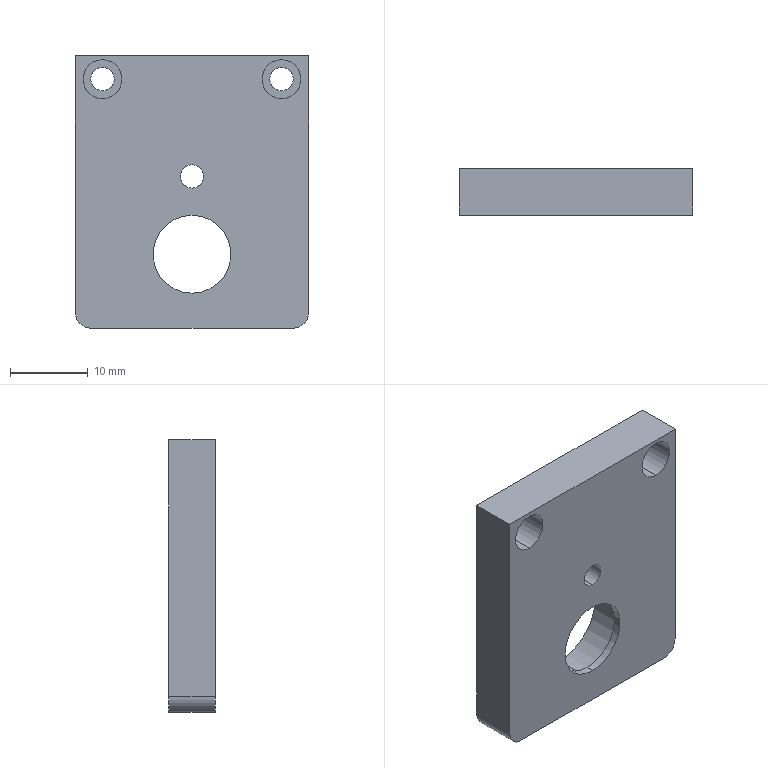Part | SolidWorks | features ICE 4, Cut 2, Extrusion 1, HoleWzd 1 | 1 solid | 33 faces | box 30 x 6 x 35 mm | volume 5244 mm3 | cylinder 20 | plane 9 | cone 4 | commonest cylinder face diameters 3 x6 2.5 x4 5 x4 4 x2 10 x2 13 x2
STEP:
#1=CARTESIAN_POINT('',(7.5,3.,3.25));
#2=VERTEX_POINT('',#1);
#3=CARTESIAN_POINT('',(7.5,3.,0.75));
#4=VERTEX_POINT('',#3);
#5=CARTESIAN_POINT('',(7.5,3.,2.));
#6=DIRECTION('',(1.,0.,0.));
#7=DIRECTION('',(0.,0.,-1.));
#8=AXIS2_PLACEMENT_3D('',#5,#6,#7);
#9=CIRCLE('',#8,1.25);
#10=EDGE_CURVE('',#2,#4,#9,.T.);
#11=ORIENTED_EDGE('',*,*,#10,.F.);
#12=CARTESIAN_POINT('',(15.,3.,3.25));
#13=VERTEX_POINT('',#12);
#14=CARTESIAN_POINT('',(15.,3.,3.25));
#15=DIRECTION('',(1.,0.,0.));
#16=VECTOR('',#15,1000.);
#17=LINE('',#14,#16);
#18=EDGE_CURVE('',#2,#13,#17,.T.);
#19=ORIENTED_EDGE('',*,*,#18,.T.);
#20=CARTESIAN_POINT('',(15.,3.,0.75));
#21=VERTEX_POINT('',#20);
#22=CARTESIAN_POINT('',(15.,3.,2.));
#23=DIRECTION('',(1.,0.,0.));
#24=DIRECTION('',(0.,0.,-1.));
#25=AXIS2_PLACEMENT_3D('',#22,#23,#24);
#26=CIRCLE('',#25,1.25);
#27=EDGE_CURVE('',#13,#21,#26,.T.);
#28=ORIENTED_EDGE('',*,*,#27,.T.);
#29=CARTESIAN_POINT('',(15.,3.,0.75));
#30=DIRECTION('',(1.,0.,0.));
#31=VECTOR('',#30,1000.);
#32=LINE('',#29,#31);
#33=EDGE_CURVE('',#4,#21,#32,.T.);
#34=ORIENTED_EDGE('',*,*,#33,.F.);
#35=EDGE_LOOP('',(#11,#19,#28,#34));
#36=FACE_OUTER_BOUND('',#35,.T.);
#37=CARTESIAN_POINT('',(15.,3.,2.));
#38=DIRECTION('',(1.,0.,0.));
#39=DIRECTION('',(0.,0.,-1.));
#40=AXIS2_PLACEMENT_3D('',#37,#38,#39);
#41=CYLINDRICAL_SURFACE('',#40,1.25);
#42=ADVANCED_FACE('',(#36),#41,.F.);
#43=CARTESIAN_POINT('',(6.749,3.,2.));
#44=VERTEX_POINT('',#43);
#45=CARTESIAN_POINT('',(7.5,3.,0.75));
#46=DIRECTION('',(0.515,0.,-0.8572));
#47=VECTOR('',#46,1000.);
#48=LINE('',#45,#47);
#49=EDGE_CURVE('',#44,#4,#48,.T.);
#50=ORIENTED_EDGE('',*,*,#49,.F.);
#51=CARTESIAN_POINT('',(7.5,3.,3.25));
#52=DIRECTION('',(0.515,0.,0.8572));
#53=VECTOR('',#52,1000.);
#54=LINE('',#51,#53);
#55=EDGE_CURVE('',#44,#2,#54,.T.);
#56=ORIENTED_EDGE('',*,*,#55,.T.);
#57=ORIENTED_EDGE('',*,*,#10,.T.);
#58=EDGE_LOOP('',(#50,#56,#57));
#59=FACE_OUTER_BOUND('',#58,.T.);
#60=CARTESIAN_POINT('',(7.5,3.,2.));
#61=DIRECTION('',(1.,0.,0.));
#62=DIRECTION('',(0.,0.,-1.));
#63=AXIS2_PLACEMENT_3D('',#60,#61,#62);
#64=CONICAL_SURFACE('',#63,1.25,1.03);
#65=ADVANCED_FACE('',(#59),#64,.F.);
#66=CARTESIAN_POINT('',(7.5,3.,-6.25));
#67=VERTEX_POINT('',#66);
#68=CARTESIAN_POINT('',(7.5,3.,-8.75));
#69=VERTEX_POINT('',#68);
#70=CARTESIAN_POINT('',(7.5,3.,-7.5));
#71=DIRECTION('',(1.,0.,0.));
#72=DIRECTION('',(0.,0.,-1.));
#73=AXIS2_PLACEMENT_3D('',#70,#71,#72);
#74=CIRCLE('',#73,1.25);
#75=EDGE_CURVE('',#67,#69,#74,.T.);
#76=ORIENTED_EDGE('',*,*,#75,.F.);
#77=CARTESIAN_POINT('',(15.,3.,-6.25));
#78=VERTEX_POINT('',#77);
#79=CARTESIAN_POINT('',(15.,3.,-6.25));
#80=DIRECTION('',(1.,0.,0.));
#81=VECTOR('',#80,1000.);
#82=LINE('',#79,#81);
#83=EDGE_CURVE('',#67,#78,#82,.T.);
#84=ORIENTED_EDGE('',*,*,#83,.T.);
#85=CARTESIAN_POINT('',(15.,3.,-8.75));
#86=VERTEX_POINT('',#85);
#87=CARTESIAN_POINT('',(15.,3.,-7.5));
#88=DIRECTION('',(1.,0.,0.));
#89=DIRECTION('',(0.,0.,-1.));
#90=AXIS2_PLACEMENT_3D('',#87,#88,#89);
#91=CIRCLE('',#90,1.25);
#92=EDGE_CURVE('',#78,#86,#91,.T.);
#93=ORIENTED_EDGE('',*,*,#92,.T.);
#94=CARTESIAN_POINT('',(15.,3.,-8.75));
#95=DIRECTION('',(1.,0.,0.));
#96=VECTOR('',#95,1000.);
#97=LINE('',#94,#96);
#98=EDGE_CURVE('',#69,#86,#97,.T.);
#99=ORIENTED_EDGE('',*,*,#98,.F.);
#100=EDGE_LOOP('',(#76,#84,#93,#99));
#101=FACE_OUTER_BOUND('',#100,.T.);
#102=CARTESIAN_POINT('',(15.,3.,-7.5));
#103=DIRECTION('',(1.,0.,0.));
#104=DIRECTION('',(0.,0.,-1.));
#105=AXIS2_PLACEMENT_3D('',#102,#103,#104);
#106=CYLINDRICAL_SURFACE('',#105,1.25);
#107=ADVANCED_FACE('',(#101),#106,.F.);
#108=CARTESIAN_POINT('',(6.749,3.,-7.5));
#109=VERTEX_POINT('',#108);
#110=CARTESIAN_POINT('',(7.5,3.,-8.75));
#111=DIRECTION('',(0.515,0.,-0.8572));
#112=VECTOR('',#111,1000.);
#113=LINE('',#110,#112);
#114=EDGE_CURVE('',#109,#69,#113,.T.);
#115=ORIENTED_EDGE('',*,*,#114,.F.);
#116=CARTESIAN_POINT('',(7.5,3.,-6.25));
#117=DIRECTION('',(0.515,0.,0.8572));
#118=VECTOR('',#117,1000.);
#119=LINE('',#116,#118);
#120=EDGE_CURVE('',#109,#67,#119,.T.);
#121=ORIENTED_EDGE('',*,*,#120,.T.);
#122=ORIENTED_EDGE('',*,*,#75,.T.);
#123=EDGE_LOOP('',(#115,#121,#122));
#124=FACE_OUTER_BOUND('',#123,.T.);
#125=CARTESIAN_POINT('',(7.5,3.,-7.5));
#126=DIRECTION('',(1.,0.,0.));
#127=DIRECTION('',(0.,0.,-1.));
#128=AXIS2_PLACEMENT_3D('',#125,#126,#127);
#129=CONICAL_SURFACE('',#128,1.25,1.03);
#130=ADVANCED_FACE('',(#124),#129,.F.);
#131=CARTESIAN_POINT('',(11.5,4.,17.));
#132=VERTEX_POINT('',#131);
#133=CARTESIAN_POINT('',(11.5,4.,12.));
#134=VERTEX_POINT('',#133);
#135=CARTESIAN_POINT('',(11.5,4.,14.5));
#136=DIRECTION('',(0.,-1.,0.));
#137=DIRECTION('',(0.,0.,-1.));
#138=AXIS2_PLACEMENT_3D('',#135,#136,#137);
#139=CIRCLE('',#138,2.5);
#140=EDGE_CURVE('',#132,#134,#139,.T.);
#141=ORIENTED_EDGE('',*,*,#140,.F.);
#142=CARTESIAN_POINT('',(11.5,0.,17.));
#143=VERTEX_POINT('',#142);
#144=CARTESIAN_POINT('',(11.5,4.,17.));
#145=DIRECTION('',(0.,-1.,0.));
#146=VECTOR('',#145,1000.);
#147=LINE('',#144,#146);
#148=EDGE_CURVE('',#132,#143,#147,.T.);
#149=ORIENTED_EDGE('',*,*,#148,.T.);
#150=CARTESIAN_POINT('',(11.5,0.,12.));
#151=VERTEX_POINT('',#150);
#152=CARTESIAN_POINT('',(11.5,0.,14.5));
#153=DIRECTION('',(0.,-1.,0.));
#154=DIRECTION('',(0.,0.,-1.));
#155=AXIS2_PLACEMENT_3D('',#152,#153,#154);
#156=CIRCLE('',#155,2.5);
#157=EDGE_CURVE('',#143,#151,#156,.T.);
#158=ORIENTED_EDGE('',*,*,#157,.T.);
#159=CARTESIAN_POINT('',(11.5,4.,12.));
#160=DIRECTION('',(0.,-1.,0.));
#161=VECTOR('',#160,1000.);
#162=LINE('',#159,#161);
#163=EDGE_CURVE('',#134,#151,#162,.T.);
#164=ORIENTED_EDGE('',*,*,#163,.F.);
#165=EDGE_LOOP('',(#141,#149,#158,#164));
#166=FACE_OUTER_BOUND('',#165,.T.);
#167=CARTESIAN_POINT('',(11.5,4.,14.5));
#168=DIRECTION('',(0.,-1.,0.));
#169=DIRECTION('',(0.,0.,-1.));
#170=AXIS2_PLACEMENT_3D('',#167,#168,#169);
#171=CYLINDRICAL_SURFACE('',#170,2.5);
#172=ADVANCED_FACE('',(#166),#171,.F.);
#173=CARTESIAN_POINT('',(-11.5,4.,17.));
#174=VERTEX_POINT('',#173);
#175=CARTESIAN_POINT('',(-11.5,4.,12.));
#176=VERTEX_POINT('',#175);
#177=CARTESIAN_POINT('',(-11.5,4.,14.5));
#178=DIRECTION('',(0.,-1.,0.));
#179=DIRECTION('',(0.,0.,-1.));
#180=AXIS2_PLACEMENT_3D('',#177,#178,#179);
#181=CIRCLE('',#180,2.5);
#182=EDGE_CURVE('',#174,#176,#181,.T.);
#183=ORIENTED_EDGE('',*,*,#182,.F.);
#184=CARTESIAN_POINT('',(-11.5,0.,17.));
#185=VERTEX_POINT('',#184);
#186=CARTESIAN_POINT('',(-11.5,4.,17.));
#187=DIRECTION('',(0.,-1.,0.));
#188=VECTOR('',#187,1000.);
#189=LINE('',#186,#188);
#190=EDGE_CURVE('',#174,#185,#189,.T.);
#191=ORIENTED_EDGE('',*,*,#190,.T.);
#192=CARTESIAN_POINT('',(-11.5,0.,12.));
#193=VERTEX_POINT('',#192);
#194=CARTESIAN_POINT('',(-11.5,0.,14.5));
#195=DIRECTION('',(0.,-1.,0.));
#196=DIRECTION('',(0.,0.,-1.));
#197=AXIS2_PLACEMENT_3D('',#194,#195,#196);
#198=CIRCLE('',#197,2.5);
#199=EDGE_CURVE('',#185,#193,#198,.T.);
#200=ORIENTED_EDGE('',*,*,#199,.T.);
#201=CARTESIAN_POINT('',(-11.5,4.,12.));
#202=DIRECTION('',(0.,-1.,0.));
#203=VECTOR('',#202,1000.);
#204=LINE('',#201,#203);
#205=EDGE_CURVE('',#176,#193,#204,.T.);
#206=ORIENTED_EDGE('',*,*,#205,.F.);
#207=EDGE_LOOP('',(#183,#191,#200,#206));
#208=FACE_OUTER_BOUND('',#207,.T.);
#209=CARTESIAN_POINT('',(-11.5,4.,14.5));
#210=DIRECTION('',(0.,-1.,0.));
#211=DIRECTION('',(0.,0.,-1.));
#212=AXIS2_PLACEMENT_3D('',#209,#210,#211);
#213=CYLINDRICAL_SURFACE('',#212,2.5);
#214=ADVANCED_FACE('',(#208),#213,.F.);
#215=CARTESIAN_POINT('',(0.,1.,-14.5));
#216=VERTEX_POINT('',#215);
#217=CARTESIAN_POINT('',(0.,1.,-1.5));
#218=VERTEX_POINT('',#217);
#219=CARTESIAN_POINT('',(0.,1.,-8.));
#220=DIRECTION('',(0.,1.,0.));
#221=DIRECTION('',(0.,0.,1.));
#222=AXIS2_PLACEMENT_3D('',#219,#220,#221);
#223=CIRCLE('',#222,6.5);
#224=EDGE_CURVE('',#216,#218,#223,.T.);
#225=ORIENTED_EDGE('',*,*,#224,.F.);
#226=CARTESIAN_POINT('',(0.,6.,-14.5));
#227=VERTEX_POINT('',#226);
#228=CARTESIAN_POINT('',(0.,1.,-14.5));
#229=DIRECTION('',(0.,1.,0.));
#230=VECTOR('',#229,1000.);
#231=LINE('',#228,#230);
#232=EDGE_CURVE('',#216,#227,#231,.T.);
#233=ORIENTED_EDGE('',*,*,#232,.T.);
#234=CARTESIAN_POINT('',(0.,6.,-1.5));
#235=VERTEX_POINT('',#234);
#236=CARTESIAN_POINT('',(0.,6.,-8.));
#237=DIRECTION('',(0.,1.,0.));
#238=DIRECTION('',(0.,0.,1.));
#239=AXIS2_PLACEMENT_3D('',#236,#237,#238);
#240=CIRCLE('',#239,6.5);
#241=EDGE_CURVE('',#227,#235,#240,.T.);
#242=ORIENTED_EDGE('',*,*,#241,.T.);
#243=CARTESIAN_POINT('',(0.,1.,-1.5));
#244=DIRECTION('',(0.,1.,0.));
#245=VECTOR('',#244,1000.);
#246=LINE('',#243,#245);
#247=EDGE_CURVE('',#218,#235,#246,.T.);
#248=ORIENTED_EDGE('',*,*,#247,.F.);
#249=EDGE_LOOP('',(#225,#233,#242,#248));
#250=FACE_OUTER_BOUND('',#249,.T.);
#251=CARTESIAN_POINT('',(0.,1.,-8.));
#252=DIRECTION('',(0.,1.,0.));
#253=DIRECTION('',(0.,0.,1.));
#254=AXIS2_PLACEMENT_3D('',#251,#252,#253);
#255=CYLINDRICAL_SURFACE('',#254,6.5);
#256=ADVANCED_FACE('',(#250),#255,.F.);
#257=CARTESIAN_POINT('',(0.,6.,0.5));
#258=VERTEX_POINT('',#257);
#259=CARTESIAN_POINT('',(0.,6.,3.5));
#260=VERTEX_POINT('',#259);
#261=CARTESIAN_POINT('',(0.,6.,2.));
#262=DIRECTION('',(0.,1.,0.));
#263=DIRECTION('',(0.,0.,1.));
#264=AXIS2_PLACEMENT_3D('',#261,#262,#263);
#265=CIRCLE('',#264,1.5);
#266=EDGE_CURVE('',#258,#260,#265,.T.);
#267=ORIENTED_EDGE('',*,*,#266,.T.);
#268=CARTESIAN_POINT('',(0.,0.,3.5));
#269=VERTEX_POINT('',#268);
#270=CARTESIAN_POINT('',(0.,6.,3.5));
#271=DIRECTION('',(0.,-1.,0.));
#272=VECTOR('',#271,1000.);
#273=LINE('',#270,#272);
#274=EDGE_CURVE('',#260,#269,#273,.T.);
#275=ORIENTED_EDGE('',*,*,#274,.T.);
#276=CARTESIAN_POINT('',(0.,0.,0.5));
#277=VERTEX_POINT('',#276);
#278=CARTESIAN_POINT('',(0.,0.,2.));
#279=DIRECTION('',(0.,1.,0.));
#280=DIRECTION('',(0.,0.,1.));
#281=AXIS2_PLACEMENT_3D('',#278,#279,#280);
#282=CIRCLE('',#281,1.5);
#283=EDGE_CURVE('',#277,#269,#282,.T.);
#284=ORIENTED_EDGE('',*,*,#283,.F.);
#285=CARTESIAN_POINT('',(0.,6.,0.5));
#286=DIRECTION('',(0.,-1.,0.));
#287=VECTOR('',#286,1000.);
#288=LINE('',#285,#287);
#289=EDGE_CURVE('',#258,#277,#288,.T.);
#290=ORIENTED_EDGE('',*,*,#289,.F.);
#291=EDGE_LOOP('',(#267,#275,#284,#290));
#292=FACE_OUTER_BOUND('',#291,.T.);
#293=CARTESIAN_POINT('',(0.,6.,2.));
#294=DIRECTION('',(0.,-1.,0.));
#295=DIRECTION('',(0.,0.,-1.));
#296=AXIS2_PLACEMENT_3D('',#293,#294,#295);
#297=CYLINDRICAL_SURFACE('',#296,1.5);
#298=ADVANCED_FACE('',(#292),#297,.F.);
#299=CARTESIAN_POINT('',(0.,1.,-13.));
#300=VERTEX_POINT('',#299);
#301=CARTESIAN_POINT('',(0.,1.,-3.));
#302=VERTEX_POINT('',#301);
#303=CARTESIAN_POINT('',(0.,1.,-8.));
#304=DIRECTION('',(0.,1.,0.));
#305=DIRECTION('',(0.,0.,1.));
#306=AXIS2_PLACEMENT_3D('',#303,#304,#305);
#307=CIRCLE('',#306,5.);
#308=EDGE_CURVE('',#300,#302,#307,.T.);
#309=ORIENTED_EDGE('',*,*,#308,.T.);
#310=CARTESIAN_POINT('',(0.,0.,-3.));
#311=VERTEX_POINT('',#310);
#312=CARTESIAN_POINT('',(0.,6.,-3.));
#313=DIRECTION('',(0.,-1.,0.));
#314=VECTOR('',#313,1000.);
#315=LINE('',#312,#314);
#316=EDGE_CURVE('',#302,#311,#315,.T.);
#317=ORIENTED_EDGE('',*,*,#316,.T.);
#318=CARTESIAN_POINT('',(0.,0.,-13.));
#319=VERTEX_POINT('',#318);
#320=CARTESIAN_POINT('',(0.,0.,-8.));
#321=DIRECTION('',(0.,1.,0.));
#322=DIRECTION('',(0.,0.,1.));
#323=AXIS2_PLACEMENT_3D('',#320,#321,#322);
#324=CIRCLE('',#323,5.);
#325=EDGE_CURVE('',#319,#311,#324,.T.);
#326=ORIENTED_EDGE('',*,*,#325,.F.);
#327=CARTESIAN_POINT('',(0.,6.,-13.));
#328=DIRECTION('',(0.,-1.,0.));
#329=VECTOR('',#328,1000.);
#330=LINE('',#327,#329);
#331=EDGE_CURVE('',#300,#319,#330,.T.);
#332=ORIENTED_EDGE('',*,*,#331,.F.);
#333=EDGE_LOOP('',(#309,#317,#326,#332));
#334=FACE_OUTER_BOUND('',#333,.T.);
#335=CARTESIAN_POINT('',(0.,6.,-8.));
#336=DIRECTION('',(0.,-1.,0.));
#337=DIRECTION('',(0.,0.,-1.));
#338=AXIS2_PLACEMENT_3D('',#335,#336,#337);
#339=CYLINDRICAL_SURFACE('',#338,5.);
#340=ADVANCED_FACE('',(#334),#339,.F.);
#341=CARTESIAN_POINT('',(-11.5,4.,13.));
#342=VERTEX_POINT('',#341);
#343=CARTESIAN_POINT('',(-11.5,4.,16.));
#344=VERTEX_POINT('',#343);
#345=CARTESIAN_POINT('',(-11.5,4.,14.5));
#346=DIRECTION('',(0.,1.,0.));
#347=DIRECTION('',(0.,0.,-1.));
#348=AXIS2_PLACEMENT_3D('',#345,#346,#347);
#349=CIRCLE('',#348,1.5);
#350=EDGE_CURVE('',#342,#344,#349,.T.);
#351=ORIENTED_EDGE('',*,*,#350,.F.);
#352=CARTESIAN_POINT('',(-11.5,6.,13.));
#353=VERTEX_POINT('',#352);
#354=CARTESIAN_POINT('',(-11.5,0.,13.));
#355=DIRECTION('',(0.,1.,0.));
#356=VECTOR('',#355,1000.);
#357=LINE('',#354,#356);
#358=EDGE_CURVE('',#342,#353,#357,.T.);
#359=ORIENTED_EDGE('',*,*,#358,.T.);
#360=CARTESIAN_POINT('',(-11.5,6.,16.));
#361=VERTEX_POINT('',#360);
#362=CARTESIAN_POINT('',(-11.5,6.,14.5));
#363=DIRECTION('',(0.,1.,0.));
#364=DIRECTION('',(0.,0.,1.));
#365=AXIS2_PLACEMENT_3D('',#362,#363,#364);
#366=CIRCLE('',#365,1.5);
#367=EDGE_CURVE('',#353,#361,#366,.T.);
#368=ORIENTED_EDGE('',*,*,#367,.T.);
#369=CARTESIAN_POINT('',(-11.5,0.,16.));
#370=DIRECTION('',(0.,1.,0.));
#371=VECTOR('',#370,1000.);
#372=LINE('',#369,#371);
#373=EDGE_CURVE('',#344,#361,#372,.T.);
#374=ORIENTED_EDGE('',*,*,#373,.F.);
#375=EDGE_LOOP('',(#351,#359,#368,#374));
#376=FACE_OUTER_BOUND('',#375,.T.);
#377=CARTESIAN_POINT('',(-11.5,0.,14.5));
#378=DIRECTION('',(0.,1.,0.));
#379=DIRECTION('',(0.,0.,1.));
#380=AXIS2_PLACEMENT_3D('',#377,#378,#379);
#381=CYLINDRICAL_SURFACE('',#380,1.5);
#382=ADVANCED_FACE('',(#376),#381,.F.);
#383=CARTESIAN_POINT('',(11.5,4.,13.));
#384=VERTEX_POINT('',#383);
#385=CARTESIAN_POINT('',(11.5,4.,16.));
#386=VERTEX_POINT('',#385);
#387=CARTESIAN_POINT('',(11.5,4.,14.5));
#388=DIRECTION('',(0.,1.,0.));
#389=DIRECTION('',(0.,0.,-1.));
#390=AXIS2_PLACEMENT_3D('',#387,#388,#389);
#391=CIRCLE('',#390,1.5);
#392=EDGE_CURVE('',#384,#386,#391,.T.);
#393=ORIENTED_EDGE('',*,*,#392,.F.);
#394=CARTESIAN_POINT('',(11.5,6.,13.));
#395=VERTEX_POINT('',#394);
#396=CARTESIAN_POINT('',(11.5,0.,13.));
#397=DIRECTION('',(0.,1.,0.));
#398=VECTOR('',#397,1000.);
#399=LINE('',#396,#398);
#400=EDGE_CURVE('',#384,#395,#399,.T.);
#401=ORIENTED_EDGE('',*,*,#400,.T.);
#402=CARTESIAN_POINT('',(11.5,6.,16.));
#403=VERTEX_POINT('',#402);
#404=CARTESIAN_POINT('',(11.5,6.,14.5));
#405=DIRECTION('',(0.,1.,0.));
#406=DIRECTION('',(0.,0.,1.));
#407=AXIS2_PLACEMENT_3D('',#404,#405,#406);
#408=CIRCLE('',#407,1.5);
#409=EDGE_CURVE('',#395,#403,#408,.T.);
#410=ORIENTED_EDGE('',*,*,#409,.T.);
#411=CARTESIAN_POINT('',(11.5,0.,16.));
#412=DIRECTION('',(0.,1.,0.));
#413=VECTOR('',#412,1000.);
#414=LINE('',#411,#413);
#415=EDGE_CURVE('',#386,#403,#414,.T.);
#416=ORIENTED_EDGE('',*,*,#415,.F.);
#417=EDGE_LOOP('',(#393,#401,#410,#416));
#418=FACE_OUTER_BOUND('',#417,.T.);
#419=CARTESIAN_POINT('',(11.5,0.,14.5));
#420=DIRECTION('',(0.,1.,0.));
#421=DIRECTION('',(0.,0.,1.));
#422=AXIS2_PLACEMENT_3D('',#419,#420,#421);
#423=CYLINDRICAL_SURFACE('',#422,1.5);
#424=ADVANCED_FACE('',(#418),#423,.F.);
#425=ORIENTED_EDGE('',*,*,#400,.F.);
#426=CARTESIAN_POINT('',(11.5,4.,14.5));
#427=DIRECTION('',(0.,1.,0.));
#428=DIRECTION('',(0.,0.,-1.));
#429=AXIS2_PLACEMENT_3D('',#426,#427,#428);
#430=CIRCLE('',#429,1.5);
#431=EDGE_CURVE('',#386,#384,#430,.T.);
#432=ORIENTED_EDGE('',*,*,#431,.F.);
#433=ORIENTED_EDGE('',*,*,#415,.T.);
#434=CARTESIAN_POINT('',(11.5,6.,14.5));
#435=DIRECTION('',(0.,1.,0.));
#436=DIRECTION('',(0.,0.,1.));
#437=AXIS2_PLACEMENT_3D('',#434,#435,#436);
#438=CIRCLE('',#437,1.5);
#439=EDGE_CURVE('',#403,#395,#438,.T.);
#440=ORIENTED_EDGE('',*,*,#439,.T.);
#441=EDGE_LOOP('',(#425,#432,#433,#440));
#442=FACE_OUTER_BOUND('',#441,.T.);
#443=CARTESIAN_POINT('',(11.5,0.,14.5));
#444=DIRECTION('',(0.,1.,0.));
#445=DIRECTION('',(0.,0.,1.));
#446=AXIS2_PLACEMENT_3D('',#443,#444,#445);
#447=CYLINDRICAL_SURFACE('',#446,1.5);
#448=ADVANCED_FACE('',(#442),#447,.F.);
#449=ORIENTED_EDGE('',*,*,#358,.F.);
#450=CARTESIAN_POINT('',(-11.5,4.,14.5));
#451=DIRECTION('',(0.,1.,0.));
#452=DIRECTION('',(0.,0.,-1.));
#453=AXIS2_PLACEMENT_3D('',#450,#451,#452);
#454=CIRCLE('',#453,1.5);
#455=EDGE_CURVE('',#344,#342,#454,.T.);
#456=ORIENTED_EDGE('',*,*,#455,.F.);
#457=ORIENTED_EDGE('',*,*,#373,.T.);
#458=CARTESIAN_POINT('',(-11.5,6.,14.5));
#459=DIRECTION('',(0.,1.,0.));
#460=DIRECTION('',(0.,0.,1.));
#461=AXIS2_PLACEMENT_3D('',#458,#459,#460);
#462=CIRCLE('',#461,1.5);
#463=EDGE_CURVE('',#361,#353,#462,.T.);
#464=ORIENTED_EDGE('',*,*,#463,.T.);
#465=EDGE_LOOP('',(#449,#456,#457,#464));
#466=FACE_OUTER_BOUND('',#465,.T.);
#467=CARTESIAN_POINT('',(-11.5,0.,14.5));
#468=DIRECTION('',(0.,1.,0.));
#469=DIRECTION('',(0.,0.,1.));
#470=AXIS2_PLACEMENT_3D('',#467,#468,#469);
#471=CYLINDRICAL_SURFACE('',#470,1.5);
#472=ADVANCED_FACE('',(#466),#471,.F.);
#473=ORIENTED_EDGE('',*,*,#316,.F.);
#474=CARTESIAN_POINT('',(0.,1.,-8.));
#475=DIRECTION('',(0.,1.,0.));
#476=DIRECTION('',(0.,0.,1.));
#477=AXIS2_PLACEMENT_3D('',#474,#475,#476);
#478=CIRCLE('',#477,5.);
#479=EDGE_CURVE('',#302,#300,#478,.T.);
#480=ORIENTED_EDGE('',*,*,#479,.T.);
#481=ORIENTED_EDGE('',*,*,#331,.T.);
#482=CARTESIAN_POINT('',(0.,0.,-8.));
#483=DIRECTION('',(0.,1.,0.));
#484=DIRECTION('',(0.,0.,1.));
#485=AXIS2_PLACEMENT_3D('',#482,#483,#484);
#486=CIRCLE('',#485,5.);
#487=EDGE_CURVE('',#311,#319,#486,.T.);
#488=ORIENTED_EDGE('',*,*,#487,.F.);
#489=EDGE_LOOP('',(#473,#480,#481,#488));
#490=FACE_OUTER_BOUND('',#489,.T.);
#491=CARTESIAN_POINT('',(0.,6.,-8.));
#492=DIRECTION('',(0.,-1.,0.));
#493=DIRECTION('',(0.,0.,-1.));
#494=AXIS2_PLACEMENT_3D('',#491,#492,#493);
#495=CYLINDRICAL_SURFACE('',#494,5.);
#496=ADVANCED_FACE('',(#490),#495,.F.);
#497=ORIENTED_EDGE('',*,*,#463,.F.);
#498=ORIENTED_EDGE('',*,*,#367,.F.);
#499=EDGE_LOOP('',(#497,#498));
#500=FACE_BOUND('',#499,.T.);
#501=ORIENTED_EDGE('',*,*,#439,.F.);
#502=ORIENTED_EDGE('',*,*,#409,.F.);
#503=EDGE_LOOP('',(#501,#502));
#504=FACE_BOUND('',#503,.T.);
#505=CARTESIAN_POINT('',(0.,6.,-8.));
#506=DIRECTION('',(0.,1.,0.));
#507=DIRECTION('',(0.,0.,1.));
#508=AXIS2_PLACEMENT_3D('',#505,#506,#507);
#509=CIRCLE('',#508,6.5);
#510=EDGE_CURVE('',#235,#227,#509,.T.);
#511=ORIENTED_EDGE('',*,*,#510,.F.);
#512=ORIENTED_EDGE('',*,*,#241,.F.);
#513=EDGE_LOOP('',(#511,#512));
#514=FACE_BOUND('',#513,.T.);
#515=CARTESIAN_POINT('',(15.,6.,-15.5));
#516=VERTEX_POINT('',#515);
#517=CARTESIAN_POINT('',(13.,6.,-17.5));
#518=VERTEX_POINT('',#517);
#519=CARTESIAN_POINT('',(13.,6.,-15.5));
#520=DIRECTION('',(0.,1.,0.));
#521=DIRECTION('',(0.,0.,-1.));
#522=AXIS2_PLACEMENT_3D('',#519,#520,#521);
#523=CIRCLE('',#522,2.);
#524=EDGE_CURVE('',#516,#518,#523,.T.);
#525=ORIENTED_EDGE('',*,*,#524,.T.);
#526=CARTESIAN_POINT('',(-13.,6.,-17.5));
#527=VERTEX_POINT('',#526);
#528=CARTESIAN_POINT('',(-13.,6.,-17.5));
#529=DIRECTION('',(-1.,0.,0.));
#530=VECTOR('',#529,1000.);
#531=LINE('',#528,#530);
#532=EDGE_CURVE('',#518,#527,#531,.T.);
#533=ORIENTED_EDGE('',*,*,#532,.T.);
#534=CARTESIAN_POINT('',(-15.,6.,-15.5));
#535=VERTEX_POINT('',#534);
#536=CARTESIAN_POINT('',(-13.,6.,-15.5));
#537=DIRECTION('',(0.,1.,0.));
#538=DIRECTION('',(0.,0.,1.));
#539=AXIS2_PLACEMENT_3D('',#536,#537,#538);
#540=CIRCLE('',#539,2.);
#541=EDGE_CURVE('',#527,#535,#540,.T.);
#542=ORIENTED_EDGE('',*,*,#541,.T.);
#543=CARTESIAN_POINT('',(-15.,6.,17.5));
#544=VERTEX_POINT('',#543);
#545=CARTESIAN_POINT('',(-15.,6.,-15.5));
#546=DIRECTION('',(0.,0.,1.));
#547=VECTOR('',#546,1000.);
#548=LINE('',#545,#547);
#549=EDGE_CURVE('',#535,#544,#548,.T.);
#550=ORIENTED_EDGE('',*,*,#549,.T.);
#551=CARTESIAN_POINT('',(15.,6.,17.5));
#552=VERTEX_POINT('',#551);
#553=CARTESIAN_POINT('',(-15.,6.,17.5));
#554=DIRECTION('',(1.,0.,0.));
#555=VECTOR('',#554,1000.);
#556=LINE('',#553,#555);
#557=EDGE_CURVE('',#544,#552,#556,.T.);
#558=ORIENTED_EDGE('',*,*,#557,.T.);
#559=CARTESIAN_POINT('',(15.,6.,-15.5));
#560=DIRECTION('',(0.,0.,-1.));
#561=VECTOR('',#560,1000.);
#562=LINE('',#559,#561);
#563=EDGE_CURVE('',#552,#516,#562,.T.);
#564=ORIENTED_EDGE('',*,*,#563,.T.);
#565=EDGE_LOOP('',(#525,#533,#542,#550,#558,#564));
#566=FACE_OUTER_BOUND('',#565,.T.);
#567=ORIENTED_EDGE('',*,*,#266,.F.);
#568=CARTESIAN_POINT('',(0.,6.,2.));
#569=DIRECTION('',(0.,1.,0.));
#570=DIRECTION('',(0.,0.,1.));
#571=AXIS2_PLACEMENT_3D('',#568,#569,#570);
#572=CIRCLE('',#571,1.5);
#573=EDGE_CURVE('',#260,#258,#572,.T.);
#574=ORIENTED_EDGE('',*,*,#573,.F.);
#575=EDGE_LOOP('',(#567,#574));
#576=FACE_BOUND('',#575,.T.);
#577=CARTESIAN_POINT('',(13.,6.,-15.5));
#578=DIRECTION('',(0.,-1.,0.));
#579=DIRECTION('',(0.,0.,-1.));
#580=AXIS2_PLACEMENT_3D('',#577,#578,#579);
#581=PLANE('',#580);
#582=ADVANCED_FACE('',(#500,#504,#514,#566,#576),#581,.F.);
#583=CARTESIAN_POINT('',(11.5,0.,14.5));
#584=DIRECTION('',(0.,-1.,0.));
#585=DIRECTION('',(0.,0.,-1.));
#586=AXIS2_PLACEMENT_3D('',#583,#584,#585);
#587=CIRCLE('',#586,2.5);
#588=EDGE_CURVE('',#151,#143,#587,.T.);
#589=ORIENTED_EDGE('',*,*,#588,.F.);
#590=ORIENTED_EDGE('',*,*,#157,.F.);
#591=EDGE_LOOP('',(#589,#590));
#592=FACE_BOUND('',#591,.T.);
#593=CARTESIAN_POINT('',(-11.5,0.,14.5));
#594=DIRECTION('',(0.,-1.,0.));
#595=DIRECTION('',(0.,0.,-1.));
#596=AXIS2_PLACEMENT_3D('',#593,#594,#595);
#597=CIRCLE('',#596,2.5);
#598=EDGE_CURVE('',#193,#185,#597,.T.);
#599=ORIENTED_EDGE('',*,*,#598,.F.);
#600=ORIENTED_EDGE('',*,*,#199,.F.);
#601=EDGE_LOOP('',(#599,#600));
#602=FACE_BOUND('',#601,.T.);
#603=ORIENTED_EDGE('',*,*,#325,.T.);
#604=ORIENTED_EDGE('',*,*,#487,.T.);
#605=EDGE_LOOP('',(#603,#604));
#606=FACE_BOUND('',#605,.T.);
#607=CARTESIAN_POINT('',(15.,0.,-15.5));
#608=VERTEX_POINT('',#607);
#609=CARTESIAN_POINT('',(13.,0.,-17.5));
#610=VERTEX_POINT('',#609);
#611=CARTESIAN_POINT('',(13.,0.,-15.5));
#612=DIRECTION('',(0.,1.,0.));
#613=DIRECTION('',(0.,0.,-1.));
#614=AXIS2_PLACEMENT_3D('',#611,#612,#613);
#615=CIRCLE('',#614,2.);
#616=EDGE_CURVE('',#608,#610,#615,.T.);
#617=ORIENTED_EDGE('',*,*,#616,.F.);
#618=CARTESIAN_POINT('',(15.,0.,17.5));
#619=VERTEX_POINT('',#618);
#620=CARTESIAN_POINT('',(15.,0.,-15.5));
#621=DIRECTION('',(0.,0.,-1.));
#622=VECTOR('',#621,1000.);
#623=LINE('',#620,#622);
#624=EDGE_CURVE('',#619,#608,#623,.T.);
#625=ORIENTED_EDGE('',*,*,#624,.F.);
#626=CARTESIAN_POINT('',(-15.,0.,17.5));
#627=VERTEX_POINT('',#626);
#628=CARTESIAN_POINT('',(-15.,0.,17.5));
#629=DIRECTION('',(1.,0.,0.));
#630=VECTOR('',#629,1000.);
#631=LINE('',#628,#630);
#632=EDGE_CURVE('',#627,#619,#631,.T.);
#633=ORIENTED_EDGE('',*,*,#632,.F.);
#634=CARTESIAN_POINT('',(-15.,0.,-15.5));
#635=VERTEX_POINT('',#634);
#636=CARTESIAN_POINT('',(-15.,0.,-15.5));
#637=DIRECTION('',(0.,0.,1.));
#638=VECTOR('',#637,1000.);
#639=LINE('',#636,#638);
#640=EDGE_CURVE('',#635,#627,#639,.T.);
#641=ORIENTED_EDGE('',*,*,#640,.F.);
#642=CARTESIAN_POINT('',(-13.,0.,-17.5));
#643=VERTEX_POINT('',#642);
#644=CARTESIAN_POINT('',(-13.,0.,-15.5));
#645=DIRECTION('',(0.,1.,0.));
#646=DIRECTION('',(0.,0.,1.));
#647=AXIS2_PLACEMENT_3D('',#644,#645,#646);
#648=CIRCLE('',#647,2.);
#649=EDGE_CURVE('',#643,#635,#648,.T.);
#650=ORIENTED_EDGE('',*,*,#649,.F.);
#651=CARTESIAN_POINT('',(-13.,0.,-17.5));
#652=DIRECTION('',(-1.,0.,0.));
#653=VECTOR('',#652,1000.);
#654=LINE('',#651,#653);
#655=EDGE_CURVE('',#610,#643,#654,.T.);
#656=ORIENTED_EDGE('',*,*,#655,.F.);
#657=EDGE_LOOP('',(#617,#625,#633,#641,#650,#656));
#658=FACE_OUTER_BOUND('',#657,.T.);
#659=ORIENTED_EDGE('',*,*,#283,.T.);
#660=CARTESIAN_POINT('',(0.,0.,2.));
#661=DIRECTION('',(0.,1.,0.));
#662=DIRECTION('',(0.,0.,1.));
#663=AXIS2_PLACEMENT_3D('',#660,#661,#662);
#664=CIRCLE('',#663,1.5);
#665=EDGE_CURVE('',#269,#277,#664,.T.);
#666=ORIENTED_EDGE('',*,*,#665,.T.);
#667=EDGE_LOOP('',(#659,#666));
#668=FACE_BOUND('',#667,.T.);
#669=CARTESIAN_POINT('',(13.,0.,-15.5));
#670=DIRECTION('',(0.,-1.,0.));
#671=DIRECTION('',(0.,0.,-1.));
#672=AXIS2_PLACEMENT_3D('',#669,#670,#671);
#673=PLANE('',#672);
#674=ADVANCED_FACE('',(#592,#602,#606,#658,#668),#673,.T.);
#675=ORIENTED_EDGE('',*,*,#616,.T.);
#676=CARTESIAN_POINT('',(13.,6.,-17.5));
#677=DIRECTION('',(0.,-1.,0.));
#678=VECTOR('',#677,1000.);
#679=LINE('',#676,#678);
#680=EDGE_CURVE('',#518,#610,#679,.T.);
#681=ORIENTED_EDGE('',*,*,#680,.F.);
#682=ORIENTED_EDGE('',*,*,#524,.F.);
#683=CARTESIAN_POINT('',(15.,6.,-15.5));
#684=DIRECTION('',(0.,-1.,0.));
#685=VECTOR('',#684,1000.);
#686=LINE('',#683,#685);
#687=EDGE_CURVE('',#516,#608,#686,.T.);
#688=ORIENTED_EDGE('',*,*,#687,.T.);
#689=EDGE_LOOP('',(#675,#681,#682,#688));
#690=FACE_OUTER_BOUND('',#689,.T.);
#691=CARTESIAN_POINT('',(13.,6.,-15.5));
#692=DIRECTION('',(0.,-1.,0.));
#693=DIRECTION('',(0.,0.,-1.));
#694=AXIS2_PLACEMENT_3D('',#691,#692,#693);
#695=CYLINDRICAL_SURFACE('',#694,2.);
#696=ADVANCED_FACE('',(#690),#695,.T.);
#697=ORIENTED_EDGE('',*,*,#655,.T.);
#698=CARTESIAN_POINT('',(-13.,6.,-17.5));
#699=DIRECTION('',(0.,-1.,0.));
#700=VECTOR('',#699,1000.);
#701=LINE('',#698,#700);
#702=EDGE_CURVE('',#527,#643,#701,.T.);
#703=ORIENTED_EDGE('',*,*,#702,.F.);
#704=ORIENTED_EDGE('',*,*,#532,.F.);
#705=ORIENTED_EDGE('',*,*,#680,.T.);
#706=EDGE_LOOP('',(#697,#703,#704,#705));
#707=FACE_OUTER_BOUND('',#706,.T.);
#708=CARTESIAN_POINT('',(-13.,6.,-17.5));
#709=DIRECTION('',(0.,0.,1.));
#710=DIRECTION('',(1.,0.,0.));
#711=AXIS2_PLACEMENT_3D('',#708,#709,#710);
#712=PLANE('',#711);
#713=ADVANCED_FACE('',(#707),#712,.F.);
#714=ORIENTED_EDGE('',*,*,#649,.T.);
#715=CARTESIAN_POINT('',(-15.,6.,-15.5));
#716=DIRECTION('',(0.,-1.,0.));
#717=VECTOR('',#716,1000.);
#718=LINE('',#715,#717);
#719=EDGE_CURVE('',#535,#635,#718,.T.);
#720=ORIENTED_EDGE('',*,*,#719,.F.);
#721=ORIENTED_EDGE('',*,*,#541,.F.);
#722=ORIENTED_EDGE('',*,*,#702,.T.);
#723=EDGE_LOOP('',(#714,#720,#721,#722));
#724=FACE_OUTER_BOUND('',#723,.T.);
#725=CARTESIAN_POINT('',(-13.,6.,-15.5));
#726=DIRECTION('',(0.,-1.,0.));
#727=DIRECTION('',(0.,0.,-1.));
#728=AXIS2_PLACEMENT_3D('',#725,#726,#727);
#729=CYLINDRICAL_SURFACE('',#728,2.);
#730=ADVANCED_FACE('',(#724),#729,.T.);
#731=ORIENTED_EDGE('',*,*,#640,.T.);
#732=CARTESIAN_POINT('',(-15.,6.,17.5));
#733=DIRECTION('',(0.,-1.,0.));
#734=VECTOR('',#733,1000.);
#735=LINE('',#732,#734);
#736=EDGE_CURVE('',#544,#627,#735,.T.);
#737=ORIENTED_EDGE('',*,*,#736,.F.);
#738=ORIENTED_EDGE('',*,*,#549,.F.);
#739=ORIENTED_EDGE('',*,*,#719,.T.);
#740=EDGE_LOOP('',(#731,#737,#738,#739));
#741=FACE_OUTER_BOUND('',#740,.T.);
#742=CARTESIAN_POINT('',(-15.,6.,-15.5));
#743=DIRECTION('',(1.,0.,0.));
#744=DIRECTION('',(0.,0.,-1.));
#745=AXIS2_PLACEMENT_3D('',#742,#743,#744);
#746=PLANE('',#745);
#747=ADVANCED_FACE('',(#741),#746,.F.);
#748=ORIENTED_EDGE('',*,*,#632,.T.);
#749=CARTESIAN_POINT('',(15.,6.,17.5));
#750=DIRECTION('',(0.,-1.,0.));
#751=VECTOR('',#750,1000.);
#752=LINE('',#749,#751);
#753=EDGE_CURVE('',#552,#619,#752,.T.);
#754=ORIENTED_EDGE('',*,*,#753,.F.);
#755=ORIENTED_EDGE('',*,*,#557,.F.);
#756=ORIENTED_EDGE('',*,*,#736,.T.);
#757=EDGE_LOOP('',(#748,#754,#755,#756));
#758=FACE_OUTER_BOUND('',#757,.T.);
#759=CARTESIAN_POINT('',(-15.,6.,17.5));
#760=DIRECTION('',(0.,0.,-1.));
#761=DIRECTION('',(-1.,0.,0.));
#762=AXIS2_PLACEMENT_3D('',#759,#760,#761);
#763=PLANE('',#762);
#764=ADVANCED_FACE('',(#758),#763,.F.);
#765=CARTESIAN_POINT('',(15.,3.,2.));
#766=DIRECTION('',(1.,0.,0.));
#767=DIRECTION('',(0.,0.,-1.));
#768=AXIS2_PLACEMENT_3D('',#765,#766,#767);
#769=CIRCLE('',#768,1.25);
#770=EDGE_CURVE('',#21,#13,#769,.T.);
#771=ORIENTED_EDGE('',*,*,#770,.F.);
#772=ORIENTED_EDGE('',*,*,#27,.F.);
#773=EDGE_LOOP('',(#771,#772));
#774=FACE_BOUND('',#773,.T.);
#775=CARTESIAN_POINT('',(15.,3.,-7.5));
#776=DIRECTION('',(1.,0.,0.));
#777=DIRECTION('',(0.,0.,-1.));
#778=AXIS2_PLACEMENT_3D('',#775,#776,#777);
#779=CIRCLE('',#778,1.25);
#780=EDGE_CURVE('',#86,#78,#779,.T.);
#781=ORIENTED_EDGE('',*,*,#780,.F.);
#782=ORIENTED_EDGE('',*,*,#92,.F.);
#783=EDGE_LOOP('',(#781,#782));
#784=FACE_BOUND('',#783,.T.);
#785=ORIENTED_EDGE('',*,*,#624,.T.);
#786=ORIENTED_EDGE('',*,*,#687,.F.);
#787=ORIENTED_EDGE('',*,*,#563,.F.);
#788=ORIENTED_EDGE('',*,*,#753,.T.);
#789=EDGE_LOOP('',(#785,#786,#787,#788));
#790=FACE_OUTER_BOUND('',#789,.T.);
#791=CARTESIAN_POINT('',(15.,6.,-15.5));
#792=DIRECTION('',(-1.,0.,0.));
#793=DIRECTION('',(0.,0.,1.));
#794=AXIS2_PLACEMENT_3D('',#791,#792,#793);
#795=PLANE('',#794);
#796=ADVANCED_FACE('',(#774,#784,#790),#795,.F.);
#797=ORIENTED_EDGE('',*,*,#274,.F.);
#798=ORIENTED_EDGE('',*,*,#573,.T.);
#799=ORIENTED_EDGE('',*,*,#289,.T.);
#800=ORIENTED_EDGE('',*,*,#665,.F.);
#801=EDGE_LOOP('',(#797,#798,#799,#800));
#802=FACE_OUTER_BOUND('',#801,.T.);
#803=CARTESIAN_POINT('',(0.,6.,2.));
#804=DIRECTION('',(0.,-1.,0.));
#805=DIRECTION('',(0.,0.,-1.));
#806=AXIS2_PLACEMENT_3D('',#803,#804,#805);
#807=CYLINDRICAL_SURFACE('',#806,1.5);
#808=ADVANCED_FACE('',(#802),#807,.F.);
#809=ORIENTED_EDGE('',*,*,#232,.F.);
#810=CARTESIAN_POINT('',(0.,1.,-8.));
#811=DIRECTION('',(0.,1.,0.));
#812=DIRECTION('',(0.,0.,1.));
#813=AXIS2_PLACEMENT_3D('',#810,#811,#812);
#814=CIRCLE('',#813,6.5);
#815=EDGE_CURVE('',#218,#216,#814,.T.);
#816=ORIENTED_EDGE('',*,*,#815,.F.);
#817=ORIENTED_EDGE('',*,*,#247,.T.);
#818=ORIENTED_EDGE('',*,*,#510,.T.);
#819=EDGE_LOOP('',(#809,#816,#817,#818));
#820=FACE_OUTER_BOUND('',#819,.T.);
#821=CARTESIAN_POINT('',(0.,1.,-8.));
#822=DIRECTION('',(0.,1.,0.));
#823=DIRECTION('',(0.,0.,1.));
#824=AXIS2_PLACEMENT_3D('',#821,#822,#823);
#825=CYLINDRICAL_SURFACE('',#824,6.5);
#826=ADVANCED_FACE('',(#820),#825,.F.);
#827=ORIENTED_EDGE('',*,*,#308,.F.);
#828=ORIENTED_EDGE('',*,*,#479,.F.);
#829=EDGE_LOOP('',(#827,#828));
#830=FACE_BOUND('',#829,.T.);
#831=ORIENTED_EDGE('',*,*,#815,.T.);
#832=ORIENTED_EDGE('',*,*,#224,.T.);
#833=EDGE_LOOP('',(#831,#832));
#834=FACE_OUTER_BOUND('',#833,.T.);
#835=CARTESIAN_POINT('',(0.,1.,-8.));
#836=DIRECTION('',(0.,1.,0.));
#837=DIRECTION('',(0.,0.,1.));
#838=AXIS2_PLACEMENT_3D('',#835,#836,#837);
#839=PLANE('',#838);
#840=ADVANCED_FACE('',(#830,#834),#839,.T.);
#841=CARTESIAN_POINT('',(-11.5,4.,14.5));
#842=DIRECTION('',(0.,-1.,0.));
#843=DIRECTION('',(0.,0.,-1.));
#844=AXIS2_PLACEMENT_3D('',#841,#842,#843);
#845=CIRCLE('',#844,2.5);
#846=EDGE_CURVE('',#176,#174,#845,.T.);
#847=ORIENTED_EDGE('',*,*,#846,.T.);
#848=ORIENTED_EDGE('',*,*,#182,.T.);
#849=EDGE_LOOP('',(#847,#848));
#850=FACE_OUTER_BOUND('',#849,.T.);
#851=ORIENTED_EDGE('',*,*,#455,.T.);
#852=ORIENTED_EDGE('',*,*,#350,.T.);
#853=EDGE_LOOP('',(#851,#852));
#854=FACE_BOUND('',#853,.T.);
#855=CARTESIAN_POINT('',(-11.5,4.,14.5));
#856=DIRECTION('',(0.,-1.,0.));
#857=DIRECTION('',(0.,0.,-1.));
#858=AXIS2_PLACEMENT_3D('',#855,#856,#857);
#859=PLANE('',#858);
#860=ADVANCED_FACE('',(#850,#854),#859,.T.);
#861=ORIENTED_EDGE('',*,*,#190,.F.);
#862=ORIENTED_EDGE('',*,*,#846,.F.);
#863=ORIENTED_EDGE('',*,*,#205,.T.);
#864=ORIENTED_EDGE('',*,*,#598,.T.);
#865=EDGE_LOOP('',(#861,#862,#863,#864));
#866=FACE_OUTER_BOUND('',#865,.T.);
#867=CARTESIAN_POINT('',(-11.5,4.,14.5));
#868=DIRECTION('',(0.,-1.,0.));
#869=DIRECTION('',(0.,0.,-1.));
#870=AXIS2_PLACEMENT_3D('',#867,#868,#869);
#871=CYLINDRICAL_SURFACE('',#870,2.5);
#872=ADVANCED_FACE('',(#866),#871,.F.);
#873=CARTESIAN_POINT('',(11.5,4.,14.5));
#874=DIRECTION('',(0.,-1.,0.));
#875=DIRECTION('',(0.,0.,-1.));
#876=AXIS2_PLACEMENT_3D('',#873,#874,#875);
#877=CIRCLE('',#876,2.5);
#878=EDGE_CURVE('',#134,#132,#877,.T.);
#879=ORIENTED_EDGE('',*,*,#878,.T.);
#880=ORIENTED_EDGE('',*,*,#140,.T.);
#881=EDGE_LOOP('',(#879,#880));
#882=FACE_OUTER_BOUND('',#881,.T.);
#883=ORIENTED_EDGE('',*,*,#431,.T.);
#884=ORIENTED_EDGE('',*,*,#392,.T.);
#885=EDGE_LOOP('',(#883,#884));
#886=FACE_BOUND('',#885,.T.);
#887=CARTESIAN_POINT('',(11.5,4.,14.5));
#888=DIRECTION('',(0.,-1.,0.));
#889=DIRECTION('',(0.,0.,-1.));
#890=AXIS2_PLACEMENT_3D('',#887,#888,#889);
#891=PLANE('',#890);
#892=ADVANCED_FACE('',(#882,#886),#891,.T.);
#893=ORIENTED_EDGE('',*,*,#148,.F.);
#894=ORIENTED_EDGE('',*,*,#878,.F.);
#895=ORIENTED_EDGE('',*,*,#163,.T.);
#896=ORIENTED_EDGE('',*,*,#588,.T.);
#897=EDGE_LOOP('',(#893,#894,#895,#896));
#898=FACE_OUTER_BOUND('',#897,.T.);
#899=CARTESIAN_POINT('',(11.5,4.,14.5));
#900=DIRECTION('',(0.,-1.,0.));
#901=DIRECTION('',(0.,0.,-1.));
#902=AXIS2_PLACEMENT_3D('',#899,#900,#901);
#903=CYLINDRICAL_SURFACE('',#902,2.5);
#904=ADVANCED_FACE('',(#898),#903,.F.);
#905=ORIENTED_EDGE('',*,*,#120,.F.);
#906=ORIENTED_EDGE('',*,*,#114,.T.);
#907=CARTESIAN_POINT('',(7.5,3.,-7.5));
#908=DIRECTION('',(1.,0.,0.));
#909=DIRECTION('',(0.,0.,-1.));
#910=AXIS2_PLACEMENT_3D('',#907,#908,#909);
#911=CIRCLE('',#910,1.25);
#912=EDGE_CURVE('',#69,#67,#911,.T.);
#913=ORIENTED_EDGE('',*,*,#912,.T.);
#914=EDGE_LOOP('',(#905,#906,#913));
#915=FACE_OUTER_BOUND('',#914,.T.);
#916=CARTESIAN_POINT('',(7.5,3.,-7.5));
#917=DIRECTION('',(1.,0.,0.));
#918=DIRECTION('',(0.,0.,-1.));
#919=AXIS2_PLACEMENT_3D('',#916,#917,#918);
#920=CONICAL_SURFACE('',#919,1.25,1.03);
#921=ADVANCED_FACE('',(#915),#920,.F.);
#922=ORIENTED_EDGE('',*,*,#83,.F.);
#923=ORIENTED_EDGE('',*,*,#912,.F.);
#924=ORIENTED_EDGE('',*,*,#98,.T.);
#925=ORIENTED_EDGE('',*,*,#780,.T.);
#926=EDGE_LOOP('',(#922,#923,#924,#925));
#927=FACE_OUTER_BOUND('',#926,.T.);
#928=CARTESIAN_POINT('',(15.,3.,-7.5));
#929=DIRECTION('',(1.,0.,0.));
#930=DIRECTION('',(0.,0.,-1.));
#931=AXIS2_PLACEMENT_3D('',#928,#929,#930);
#932=CYLINDRICAL_SURFACE('',#931,1.25);
#933=ADVANCED_FACE('',(#927),#932,.F.);
#934=ORIENTED_EDGE('',*,*,#55,.F.);
#935=ORIENTED_EDGE('',*,*,#49,.T.);
#936=CARTESIAN_POINT('',(7.5,3.,2.));
#937=DIRECTION('',(1.,0.,0.));
#938=DIRECTION('',(0.,0.,-1.));
#939=AXIS2_PLACEMENT_3D('',#936,#937,#938);
#940=CIRCLE('',#939,1.25);
#941=EDGE_CURVE('',#4,#2,#940,.T.);
#942=ORIENTED_EDGE('',*,*,#941,.T.);
#943=EDGE_LOOP('',(#934,#935,#942));
#944=FACE_OUTER_BOUND('',#943,.T.);
#945=CARTESIAN_POINT('',(7.5,3.,2.));
#946=DIRECTION('',(1.,0.,0.));
#947=DIRECTION('',(0.,0.,-1.));
#948=AXIS2_PLACEMENT_3D('',#945,#946,#947);
#949=CONICAL_SURFACE('',#948,1.25,1.03);
#950=ADVANCED_FACE('',(#944),#949,.F.);
#951=ORIENTED_EDGE('',*,*,#18,.F.);
#952=ORIENTED_EDGE('',*,*,#941,.F.);
#953=ORIENTED_EDGE('',*,*,#33,.T.);
#954=ORIENTED_EDGE('',*,*,#770,.T.);
#955=EDGE_LOOP('',(#951,#952,#953,#954));
#956=FACE_OUTER_BOUND('',#955,.T.);
#957=CARTESIAN_POINT('',(15.,3.,2.));
#958=DIRECTION('',(1.,0.,0.));
#959=DIRECTION('',(0.,0.,-1.));
#960=AXIS2_PLACEMENT_3D('',#957,#958,#959);
#961=CYLINDRICAL_SURFACE('',#960,1.25);
#962=ADVANCED_FACE('',(#956),#961,.F.);
#963=CLOSED_SHELL('',(#42,#65,#107,#130,#172,#214,#256,#298,#340,#382,#424,#448,#472,#496,#582,#674,#696,#713,#730,#747,#764,#796,#808,#826,#840,#860,#872,#892,#904,#921,#933,#950,#962));
#964=MANIFOLD_SOLID_BREP('',#963);
#965=CARTESIAN_POINT('',(0.,0.,0.));
#966=DIRECTION('',(0.,0.,1.));
#967=DIRECTION('',(1.,0.,0.));
#968=AXIS2_PLACEMENT_3D('',#965,#966,#967);
#969=(LENGTH_UNIT()NAMED_UNIT(*)SI_UNIT(.MILLI.,.METRE.));
#970=UNCERTAINTY_MEASURE_WITH_UNIT(LENGTH_MEASURE(0.00001),#969,'','');
#971=(NAMED_UNIT(*)PLANE_ANGLE_UNIT()SI_UNIT($,.RADIAN.));
#972=(NAMED_UNIT(*)SI_UNIT($,.STERADIAN.)SOLID_ANGLE_UNIT());
#973=(GEOMETRIC_REPRESENTATION_CONTEXT(3)GLOBAL_UNCERTAINTY_ASSIGNED_CONTEXT((#970))GLOBAL_UNIT_ASSIGNED_CONTEXT((#969,#971,#972))REPRESENTATION_CONTEXT('',''));
#974=ADVANCED_BREP_SHAPE_REPRESENTATION('',(#964,#968),#973);